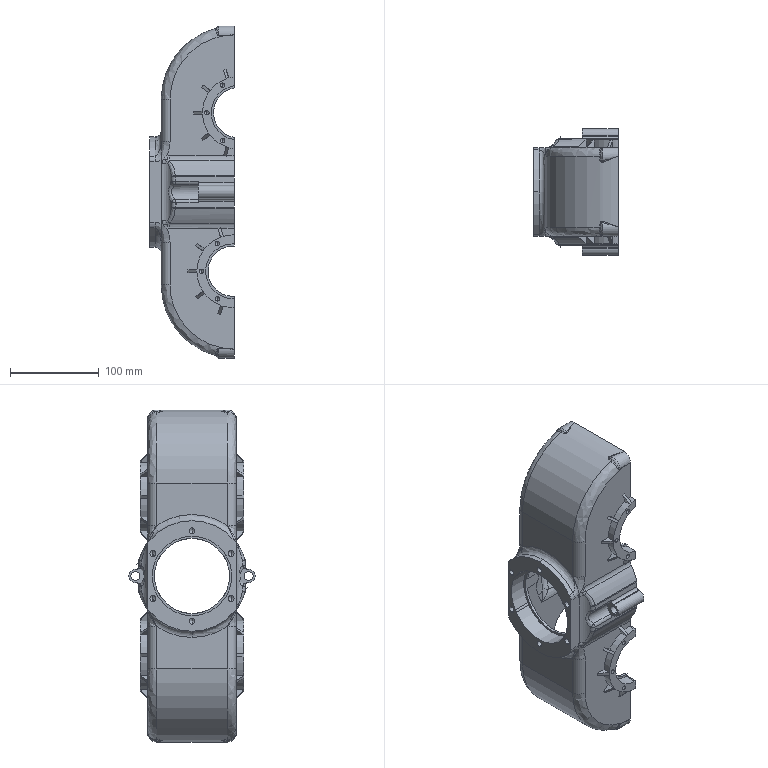Part | SolidWorks | features BaseBody 3 | 3 solids | 405 faces | box 95.5 x 143.009 x 375 mm | volume 821639 mm3 | cylinder 172 | plane 108 | spline 70 | cone 44 | sphere 8 | torus 3 | commonest cylinder face diameters 20 x26 82 x26 5 x24 10 x13 6.8 x12 10.2 x12